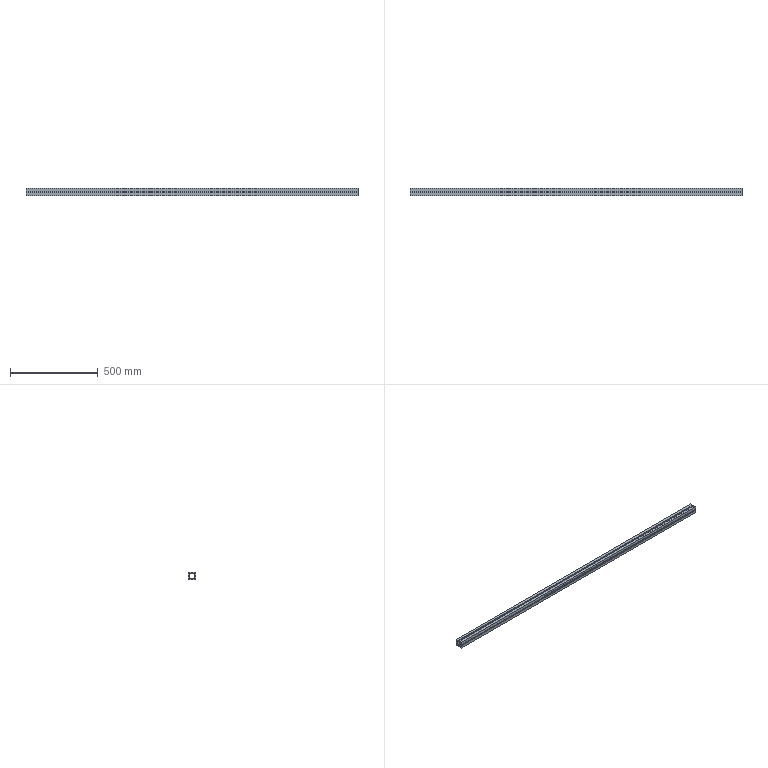Part | SolidWorks | features Extrusion 1 | 1 solid | 42 faces | box 1890 x 40 x 40 mm | volume 1315440 mm3 | plane 42
STEP:
#1=CARTESIAN_POINT('',(1890.,3.,-20.));
#2=VERTEX_POINT('',#1);
#3=CARTESIAN_POINT('',(1890.,20.,-20.));
#4=VERTEX_POINT('',#3);
#5=CARTESIAN_POINT('',(1890.,3.,-20.));
#6=DIRECTION('',(0.,1.,0.));
#7=VECTOR('',#6,1000.);
#8=LINE('',#5,#7);
#9=EDGE_CURVE('',#2,#4,#8,.T.);
#10=ORIENTED_EDGE('',*,*,#9,.T.);
#11=CARTESIAN_POINT('',(1890.,20.,-3.));
#12=VERTEX_POINT('',#11);
#13=CARTESIAN_POINT('',(1890.,20.,-3.));
#14=DIRECTION('',(0.,0.,1.));
#15=VECTOR('',#14,1000.);
#16=LINE('',#13,#15);
#17=EDGE_CURVE('',#4,#12,#16,.T.);
#18=ORIENTED_EDGE('',*,*,#17,.T.);
#19=CARTESIAN_POINT('',(1890.,17.,-3.));
#20=VERTEX_POINT('',#19);
#21=CARTESIAN_POINT('',(1890.,20.,-3.));
#22=DIRECTION('',(0.,-1.,0.));
#23=VECTOR('',#22,1000.);
#24=LINE('',#21,#23);
#25=EDGE_CURVE('',#12,#20,#24,.T.);
#26=ORIENTED_EDGE('',*,*,#25,.T.);
#27=CARTESIAN_POINT('',(1890.,17.,-6.5));
#28=VERTEX_POINT('',#27);
#29=CARTESIAN_POINT('',(1890.,17.,-3.));
#30=DIRECTION('',(0.,0.,-1.));
#31=VECTOR('',#30,1000.);
#32=LINE('',#29,#31);
#33=EDGE_CURVE('',#20,#28,#32,.T.);
#34=ORIENTED_EDGE('',*,*,#33,.T.);
#35=CARTESIAN_POINT('',(1890.,14.,-6.5));
#36=VERTEX_POINT('',#35);
#37=CARTESIAN_POINT('',(1890.,17.,-6.5));
#38=DIRECTION('',(0.,-1.,0.));
#39=VECTOR('',#38,1000.);
#40=LINE('',#37,#39);
#41=EDGE_CURVE('',#28,#36,#40,.T.);
#42=ORIENTED_EDGE('',*,*,#41,.T.);
#43=CARTESIAN_POINT('',(1890.,14.,6.5));
#44=VERTEX_POINT('',#43);
#45=CARTESIAN_POINT('',(1890.,14.,6.5));
#46=DIRECTION('',(0.,0.,1.));
#47=VECTOR('',#46,1000.);
#48=LINE('',#45,#47);
#49=EDGE_CURVE('',#36,#44,#48,.T.);
#50=ORIENTED_EDGE('',*,*,#49,.T.);
#51=CARTESIAN_POINT('',(1890.,17.,6.5));
#52=VERTEX_POINT('',#51);
#53=CARTESIAN_POINT('',(1890.,17.,6.5));
#54=DIRECTION('',(0.,1.,0.));
#55=VECTOR('',#54,1000.);
#56=LINE('',#53,#55);
#57=EDGE_CURVE('',#44,#52,#56,.T.);
#58=ORIENTED_EDGE('',*,*,#57,.T.);
#59=CARTESIAN_POINT('',(1890.,17.,3.));
#60=VERTEX_POINT('',#59);
#61=CARTESIAN_POINT('',(1890.,17.,6.5));
#62=DIRECTION('',(0.,0.,-1.));
#63=VECTOR('',#62,1000.);
#64=LINE('',#61,#63);
#65=EDGE_CURVE('',#52,#60,#64,.T.);
#66=ORIENTED_EDGE('',*,*,#65,.T.);
#67=CARTESIAN_POINT('',(1890.,20.,3.));
#68=VERTEX_POINT('',#67);
#69=CARTESIAN_POINT('',(1890.,20.,3.));
#70=DIRECTION('',(0.,1.,0.));
#71=VECTOR('',#70,1000.);
#72=LINE('',#69,#71);
#73=EDGE_CURVE('',#60,#68,#72,.T.);
#74=ORIENTED_EDGE('',*,*,#73,.T.);
#75=CARTESIAN_POINT('',(1890.,20.,20.));
#76=VERTEX_POINT('',#75);
#77=CARTESIAN_POINT('',(1890.,20.,20.));
#78=DIRECTION('',(0.,0.,1.));
#79=VECTOR('',#78,1000.);
#80=LINE('',#77,#79);
#81=EDGE_CURVE('',#68,#76,#80,.T.);
#82=ORIENTED_EDGE('',*,*,#81,.T.);
#83=CARTESIAN_POINT('',(1890.,3.,20.));
#84=VERTEX_POINT('',#83);
#85=CARTESIAN_POINT('',(1890.,3.,20.));
#86=DIRECTION('',(0.,-1.,0.));
#87=VECTOR('',#86,1000.);
#88=LINE('',#85,#87);
#89=EDGE_CURVE('',#76,#84,#88,.T.);
#90=ORIENTED_EDGE('',*,*,#89,.T.);
#91=CARTESIAN_POINT('',(1890.,3.,17.));
#92=VERTEX_POINT('',#91);
#93=CARTESIAN_POINT('',(1890.,3.,17.));
#94=DIRECTION('',(0.,0.,-1.));
#95=VECTOR('',#94,1000.);
#96=LINE('',#93,#95);
#97=EDGE_CURVE('',#84,#92,#96,.T.);
#98=ORIENTED_EDGE('',*,*,#97,.T.);
#99=CARTESIAN_POINT('',(1890.,6.5,17.));
#100=VERTEX_POINT('',#99);
#101=CARTESIAN_POINT('',(1890.,3.,17.));
#102=DIRECTION('',(0.,1.,0.));
#103=VECTOR('',#102,1000.);
#104=LINE('',#101,#103);
#105=EDGE_CURVE('',#92,#100,#104,.T.);
#106=ORIENTED_EDGE('',*,*,#105,.T.);
#107=CARTESIAN_POINT('',(1890.,6.5,14.));
#108=VERTEX_POINT('',#107);
#109=CARTESIAN_POINT('',(1890.,6.5,14.));
#110=DIRECTION('',(0.,0.,-1.));
#111=VECTOR('',#110,1000.);
#112=LINE('',#109,#111);
#113=EDGE_CURVE('',#100,#108,#112,.T.);
#114=ORIENTED_EDGE('',*,*,#113,.T.);
#115=CARTESIAN_POINT('',(1890.,-6.5,14.));
#116=VERTEX_POINT('',#115);
#117=CARTESIAN_POINT('',(1890.,-6.5,14.));
#118=DIRECTION('',(0.,-1.,0.));
#119=VECTOR('',#118,1000.);
#120=LINE('',#117,#119);
#121=EDGE_CURVE('',#108,#116,#120,.T.);
#122=ORIENTED_EDGE('',*,*,#121,.T.);
#123=CARTESIAN_POINT('',(1890.,-6.5,17.));
#124=VERTEX_POINT('',#123);
#125=CARTESIAN_POINT('',(1890.,-6.5,14.));
#126=DIRECTION('',(0.,0.,1.));
#127=VECTOR('',#126,1000.);
#128=LINE('',#125,#127);
#129=EDGE_CURVE('',#116,#124,#128,.T.);
#130=ORIENTED_EDGE('',*,*,#129,.T.);
#131=CARTESIAN_POINT('',(1890.,-3.,17.));
#132=VERTEX_POINT('',#131);
#133=CARTESIAN_POINT('',(1890.,-6.5,17.));
#134=DIRECTION('',(0.,1.,0.));
#135=VECTOR('',#134,1000.);
#136=LINE('',#133,#135);
#137=EDGE_CURVE('',#124,#132,#136,.T.);
#138=ORIENTED_EDGE('',*,*,#137,.T.);
#139=CARTESIAN_POINT('',(1890.,-3.,20.));
#140=VERTEX_POINT('',#139);
#141=CARTESIAN_POINT('',(1890.,-3.,17.));
#142=DIRECTION('',(0.,0.,1.));
#143=VECTOR('',#142,1000.);
#144=LINE('',#141,#143);
#145=EDGE_CURVE('',#132,#140,#144,.T.);
#146=ORIENTED_EDGE('',*,*,#145,.T.);
#147=CARTESIAN_POINT('',(1890.,-20.,20.));
#148=VERTEX_POINT('',#147);
#149=CARTESIAN_POINT('',(1890.,-20.,20.));
#150=DIRECTION('',(0.,-1.,0.));
#151=VECTOR('',#150,1000.);
#152=LINE('',#149,#151);
#153=EDGE_CURVE('',#140,#148,#152,.T.);
#154=ORIENTED_EDGE('',*,*,#153,.T.);
#155=CARTESIAN_POINT('',(1890.,-20.,3.));
#156=VERTEX_POINT('',#155);
#157=CARTESIAN_POINT('',(1890.,-20.,20.));
#158=DIRECTION('',(0.,0.,-1.));
#159=VECTOR('',#158,1000.);
#160=LINE('',#157,#159);
#161=EDGE_CURVE('',#148,#156,#160,.T.);
#162=ORIENTED_EDGE('',*,*,#161,.T.);
#163=CARTESIAN_POINT('',(1890.,-17.,3.));
#164=VERTEX_POINT('',#163);
#165=CARTESIAN_POINT('',(1890.,-20.,3.));
#166=DIRECTION('',(0.,1.,0.));
#167=VECTOR('',#166,1000.);
#168=LINE('',#165,#167);
#169=EDGE_CURVE('',#156,#164,#168,.T.);
#170=ORIENTED_EDGE('',*,*,#169,.T.);
#171=CARTESIAN_POINT('',(1890.,-17.,6.5));
#172=VERTEX_POINT('',#171);
#173=CARTESIAN_POINT('',(1890.,-17.,6.5));
#174=DIRECTION('',(0.,0.,1.));
#175=VECTOR('',#174,1000.);
#176=LINE('',#173,#175);
#177=EDGE_CURVE('',#164,#172,#176,.T.);
#178=ORIENTED_EDGE('',*,*,#177,.T.);
#179=CARTESIAN_POINT('',(1890.,-14.,6.5));
#180=VERTEX_POINT('',#179);
#181=CARTESIAN_POINT('',(1890.,-17.,6.5));
#182=DIRECTION('',(0.,1.,0.));
#183=VECTOR('',#182,1000.);
#184=LINE('',#181,#183);
#185=EDGE_CURVE('',#172,#180,#184,.T.);
#186=ORIENTED_EDGE('',*,*,#185,.T.);
#187=CARTESIAN_POINT('',(1890.,-14.,-6.5));
#188=VERTEX_POINT('',#187);
#189=CARTESIAN_POINT('',(1890.,-14.,6.5));
#190=DIRECTION('',(0.,0.,-1.));
#191=VECTOR('',#190,1000.);
#192=LINE('',#189,#191);
#193=EDGE_CURVE('',#180,#188,#192,.T.);
#194=ORIENTED_EDGE('',*,*,#193,.T.);
#195=CARTESIAN_POINT('',(1890.,-17.,-6.5));
#196=VERTEX_POINT('',#195);
#197=CARTESIAN_POINT('',(1890.,-17.,-6.5));
#198=DIRECTION('',(0.,-1.,0.));
#199=VECTOR('',#198,1000.);
#200=LINE('',#197,#199);
#201=EDGE_CURVE('',#188,#196,#200,.T.);
#202=ORIENTED_EDGE('',*,*,#201,.T.);
#203=CARTESIAN_POINT('',(1890.,-17.,-3.));
#204=VERTEX_POINT('',#203);
#205=CARTESIAN_POINT('',(1890.,-17.,-3.));
#206=DIRECTION('',(0.,0.,1.));
#207=VECTOR('',#206,1000.);
#208=LINE('',#205,#207);
#209=EDGE_CURVE('',#196,#204,#208,.T.);
#210=ORIENTED_EDGE('',*,*,#209,.T.);
#211=CARTESIAN_POINT('',(1890.,-20.,-3.));
#212=VERTEX_POINT('',#211);
#213=CARTESIAN_POINT('',(1890.,-20.,-3.));
#214=DIRECTION('',(0.,-1.,0.));
#215=VECTOR('',#214,1000.);
#216=LINE('',#213,#215);
#217=EDGE_CURVE('',#204,#212,#216,.T.);
#218=ORIENTED_EDGE('',*,*,#217,.T.);
#219=CARTESIAN_POINT('',(1890.,-20.,-20.));
#220=VERTEX_POINT('',#219);
#221=CARTESIAN_POINT('',(1890.,-20.,-3.));
#222=DIRECTION('',(0.,0.,-1.));
#223=VECTOR('',#222,1000.);
#224=LINE('',#221,#223);
#225=EDGE_CURVE('',#212,#220,#224,.T.);
#226=ORIENTED_EDGE('',*,*,#225,.T.);
#227=CARTESIAN_POINT('',(1890.,-3.,-20.));
#228=VERTEX_POINT('',#227);
#229=CARTESIAN_POINT('',(1890.,-20.,-20.));
#230=DIRECTION('',(0.,1.,0.));
#231=VECTOR('',#230,1000.);
#232=LINE('',#229,#231);
#233=EDGE_CURVE('',#220,#228,#232,.T.);
#234=ORIENTED_EDGE('',*,*,#233,.T.);
#235=CARTESIAN_POINT('',(1890.,-3.,-17.));
#236=VERTEX_POINT('',#235);
#237=CARTESIAN_POINT('',(1890.,-3.,-17.));
#238=DIRECTION('',(0.,0.,1.));
#239=VECTOR('',#238,1000.);
#240=LINE('',#237,#239);
#241=EDGE_CURVE('',#228,#236,#240,.T.);
#242=ORIENTED_EDGE('',*,*,#241,.T.);
#243=CARTESIAN_POINT('',(1890.,-6.5,-17.));
#244=VERTEX_POINT('',#243);
#245=CARTESIAN_POINT('',(1890.,-6.5,-17.));
#246=DIRECTION('',(0.,-1.,0.));
#247=VECTOR('',#246,1000.);
#248=LINE('',#245,#247);
#249=EDGE_CURVE('',#236,#244,#248,.T.);
#250=ORIENTED_EDGE('',*,*,#249,.T.);
#251=CARTESIAN_POINT('',(1890.,-6.5,-14.));
#252=VERTEX_POINT('',#251);
#253=CARTESIAN_POINT('',(1890.,-6.5,-14.));
#254=DIRECTION('',(0.,0.,1.));
#255=VECTOR('',#254,1000.);
#256=LINE('',#253,#255);
#257=EDGE_CURVE('',#244,#252,#256,.T.);
#258=ORIENTED_EDGE('',*,*,#257,.T.);
#259=CARTESIAN_POINT('',(1890.,6.5,-14.));
#260=VERTEX_POINT('',#259);
#261=CARTESIAN_POINT('',(1890.,-6.5,-14.));
#262=DIRECTION('',(0.,1.,0.));
#263=VECTOR('',#262,1000.);
#264=LINE('',#261,#263);
#265=EDGE_CURVE('',#252,#260,#264,.T.);
#266=ORIENTED_EDGE('',*,*,#265,.T.);
#267=CARTESIAN_POINT('',(1890.,6.5,-17.));
#268=VERTEX_POINT('',#267);
#269=CARTESIAN_POINT('',(1890.,6.5,-14.));
#270=DIRECTION('',(0.,0.,-1.));
#271=VECTOR('',#270,1000.);
#272=LINE('',#269,#271);
#273=EDGE_CURVE('',#260,#268,#272,.T.);
#274=ORIENTED_EDGE('',*,*,#273,.T.);
#275=CARTESIAN_POINT('',(1890.,3.,-17.));
#276=VERTEX_POINT('',#275);
#277=CARTESIAN_POINT('',(1890.,3.,-17.));
#278=DIRECTION('',(0.,-1.,0.));
#279=VECTOR('',#278,1000.);
#280=LINE('',#277,#279);
#281=EDGE_CURVE('',#268,#276,#280,.T.);
#282=ORIENTED_EDGE('',*,*,#281,.T.);
#283=CARTESIAN_POINT('',(1890.,3.,-17.));
#284=DIRECTION('',(0.,0.,-1.));
#285=VECTOR('',#284,1000.);
#286=LINE('',#283,#285);
#287=EDGE_CURVE('',#276,#2,#286,.T.);
#288=ORIENTED_EDGE('',*,*,#287,.T.);
#289=EDGE_LOOP('',(#10,#18,#26,#34,#42,#50,#58,#66,#74,#82,#90,#98,#106,#114,#122,#130,#138,#146,#154,#162,#170,#178,#186,#194,#202,#210,#218,#226,#234,#242,#250,#258,#266,#274,#282,#288));
#290=FACE_OUTER_BOUND('',#289,.T.);
#291=CARTESIAN_POINT('',(1890.,-13.,-13.));
#292=VERTEX_POINT('',#291);
#293=CARTESIAN_POINT('',(1890.,13.,-13.));
#294=VERTEX_POINT('',#293);
#295=CARTESIAN_POINT('',(1890.,-13.,-13.));
#296=DIRECTION('',(0.,1.,0.));
#297=VECTOR('',#296,1000.);
#298=LINE('',#295,#297);
#299=EDGE_CURVE('',#292,#294,#298,.T.);
#300=ORIENTED_EDGE('',*,*,#299,.F.);
#301=CARTESIAN_POINT('',(1890.,-13.,13.));
#302=VERTEX_POINT('',#301);
#303=CARTESIAN_POINT('',(1890.,-13.,13.));
#304=DIRECTION('',(0.,0.,-1.));
#305=VECTOR('',#304,1000.);
#306=LINE('',#303,#305);
#307=EDGE_CURVE('',#302,#292,#306,.T.);
#308=ORIENTED_EDGE('',*,*,#307,.F.);
#309=CARTESIAN_POINT('',(1890.,13.,13.));
#310=VERTEX_POINT('',#309);
#311=CARTESIAN_POINT('',(1890.,-13.,13.));
#312=DIRECTION('',(0.,-1.,0.));
#313=VECTOR('',#312,1000.);
#314=LINE('',#311,#313);
#315=EDGE_CURVE('',#310,#302,#314,.T.);
#316=ORIENTED_EDGE('',*,*,#315,.F.);
#317=CARTESIAN_POINT('',(1890.,13.,13.));
#318=DIRECTION('',(0.,0.,1.));
#319=VECTOR('',#318,1000.);
#320=LINE('',#317,#319);
#321=EDGE_CURVE('',#294,#310,#320,.T.);
#322=ORIENTED_EDGE('',*,*,#321,.F.);
#323=EDGE_LOOP('',(#300,#308,#316,#322));
#324=FACE_BOUND('',#323,.T.);
#325=CARTESIAN_POINT('',(1890.,20.,-20.));
#326=DIRECTION('',(-1.,0.,0.));
#327=DIRECTION('',(0.,0.,1.));
#328=AXIS2_PLACEMENT_3D('',#325,#326,#327);
#329=PLANE('',#328);
#330=ADVANCED_FACE('',(#290,#324),#329,.F.);
#331=CARTESIAN_POINT('',(0.,3.,-20.));
#332=VERTEX_POINT('',#331);
#333=CARTESIAN_POINT('',(0.,20.,-20.));
#334=VERTEX_POINT('',#333);
#335=CARTESIAN_POINT('',(0.,3.,-20.));
#336=DIRECTION('',(0.,1.,0.));
#337=VECTOR('',#336,1000.);
#338=LINE('',#335,#337);
#339=EDGE_CURVE('',#332,#334,#338,.T.);
#340=ORIENTED_EDGE('',*,*,#339,.F.);
#341=CARTESIAN_POINT('',(0.,3.,-17.));
#342=VERTEX_POINT('',#341);
#343=CARTESIAN_POINT('',(0.,3.,-17.));
#344=DIRECTION('',(0.,0.,-1.));
#345=VECTOR('',#344,1000.);
#346=LINE('',#343,#345);
#347=EDGE_CURVE('',#342,#332,#346,.T.);
#348=ORIENTED_EDGE('',*,*,#347,.F.);
#349=CARTESIAN_POINT('',(0.,6.5,-17.));
#350=VERTEX_POINT('',#349);
#351=CARTESIAN_POINT('',(0.,3.,-17.));
#352=DIRECTION('',(0.,-1.,0.));
#353=VECTOR('',#352,1000.);
#354=LINE('',#351,#353);
#355=EDGE_CURVE('',#350,#342,#354,.T.);
#356=ORIENTED_EDGE('',*,*,#355,.F.);
#357=CARTESIAN_POINT('',(0.,6.5,-14.));
#358=VERTEX_POINT('',#357);
#359=CARTESIAN_POINT('',(0.,6.5,-14.));
#360=DIRECTION('',(0.,0.,-1.));
#361=VECTOR('',#360,1000.);
#362=LINE('',#359,#361);
#363=EDGE_CURVE('',#358,#350,#362,.T.);
#364=ORIENTED_EDGE('',*,*,#363,.F.);
#365=CARTESIAN_POINT('',(0.,-6.5,-14.));
#366=VERTEX_POINT('',#365);
#367=CARTESIAN_POINT('',(0.,-6.5,-14.));
#368=DIRECTION('',(0.,1.,0.));
#369=VECTOR('',#368,1000.);
#370=LINE('',#367,#369);
#371=EDGE_CURVE('',#366,#358,#370,.T.);
#372=ORIENTED_EDGE('',*,*,#371,.F.);
#373=CARTESIAN_POINT('',(0.,-6.5,-17.));
#374=VERTEX_POINT('',#373);
#375=CARTESIAN_POINT('',(0.,-6.5,-14.));
#376=DIRECTION('',(0.,0.,1.));
#377=VECTOR('',#376,1000.);
#378=LINE('',#375,#377);
#379=EDGE_CURVE('',#374,#366,#378,.T.);
#380=ORIENTED_EDGE('',*,*,#379,.F.);
#381=CARTESIAN_POINT('',(0.,-3.,-17.));
#382=VERTEX_POINT('',#381);
#383=CARTESIAN_POINT('',(0.,-6.5,-17.));
#384=DIRECTION('',(0.,-1.,0.));
#385=VECTOR('',#384,1000.);
#386=LINE('',#383,#385);
#387=EDGE_CURVE('',#382,#374,#386,.T.);
#388=ORIENTED_EDGE('',*,*,#387,.F.);
#389=CARTESIAN_POINT('',(0.,-3.,-20.));
#390=VERTEX_POINT('',#389);
#391=CARTESIAN_POINT('',(0.,-3.,-17.));
#392=DIRECTION('',(0.,0.,1.));
#393=VECTOR('',#392,1000.);
#394=LINE('',#391,#393);
#395=EDGE_CURVE('',#390,#382,#394,.T.);
#396=ORIENTED_EDGE('',*,*,#395,.F.);
#397=CARTESIAN_POINT('',(0.,-20.,-20.));
#398=VERTEX_POINT('',#397);
#399=CARTESIAN_POINT('',(0.,-20.,-20.));
#400=DIRECTION('',(0.,1.,0.));
#401=VECTOR('',#400,1000.);
#402=LINE('',#399,#401);
#403=EDGE_CURVE('',#398,#390,#402,.T.);
#404=ORIENTED_EDGE('',*,*,#403,.F.);
#405=CARTESIAN_POINT('',(0.,-20.,-3.));
#406=VERTEX_POINT('',#405);
#407=CARTESIAN_POINT('',(0.,-20.,-3.));
#408=DIRECTION('',(0.,0.,-1.));
#409=VECTOR('',#408,1000.);
#410=LINE('',#407,#409);
#411=EDGE_CURVE('',#406,#398,#410,.T.);
#412=ORIENTED_EDGE('',*,*,#411,.F.);
#413=CARTESIAN_POINT('',(0.,-17.,-3.));
#414=VERTEX_POINT('',#413);
#415=CARTESIAN_POINT('',(0.,-20.,-3.));
#416=DIRECTION('',(0.,-1.,0.));
#417=VECTOR('',#416,1000.);
#418=LINE('',#415,#417);
#419=EDGE_CURVE('',#414,#406,#418,.T.);
#420=ORIENTED_EDGE('',*,*,#419,.F.);
#421=CARTESIAN_POINT('',(0.,-17.,-6.5));
#422=VERTEX_POINT('',#421);
#423=CARTESIAN_POINT('',(0.,-17.,-3.));
#424=DIRECTION('',(0.,0.,1.));
#425=VECTOR('',#424,1000.);
#426=LINE('',#423,#425);
#427=EDGE_CURVE('',#422,#414,#426,.T.);
#428=ORIENTED_EDGE('',*,*,#427,.F.);
#429=CARTESIAN_POINT('',(0.,-14.,-6.5));
#430=VERTEX_POINT('',#429);
#431=CARTESIAN_POINT('',(0.,-17.,-6.5));
#432=DIRECTION('',(0.,-1.,0.));
#433=VECTOR('',#432,1000.);
#434=LINE('',#431,#433);
#435=EDGE_CURVE('',#430,#422,#434,.T.);
#436=ORIENTED_EDGE('',*,*,#435,.F.);
#437=CARTESIAN_POINT('',(0.,-14.,6.5));
#438=VERTEX_POINT('',#437);
#439=CARTESIAN_POINT('',(0.,-14.,6.5));
#440=DIRECTION('',(0.,0.,-1.));
#441=VECTOR('',#440,1000.);
#442=LINE('',#439,#441);
#443=EDGE_CURVE('',#438,#430,#442,.T.);
#444=ORIENTED_EDGE('',*,*,#443,.F.);
#445=CARTESIAN_POINT('',(0.,-17.,6.5));
#446=VERTEX_POINT('',#445);
#447=CARTESIAN_POINT('',(0.,-17.,6.5));
#448=DIRECTION('',(0.,1.,0.));
#449=VECTOR('',#448,1000.);
#450=LINE('',#447,#449);
#451=EDGE_CURVE('',#446,#438,#450,.T.);
#452=ORIENTED_EDGE('',*,*,#451,.F.);
#453=CARTESIAN_POINT('',(0.,-17.,3.));
#454=VERTEX_POINT('',#453);
#455=CARTESIAN_POINT('',(0.,-17.,6.5));
#456=DIRECTION('',(0.,0.,1.));
#457=VECTOR('',#456,1000.);
#458=LINE('',#455,#457);
#459=EDGE_CURVE('',#454,#446,#458,.T.);
#460=ORIENTED_EDGE('',*,*,#459,.F.);
#461=CARTESIAN_POINT('',(0.,-20.,3.));
#462=VERTEX_POINT('',#461);
#463=CARTESIAN_POINT('',(0.,-20.,3.));
#464=DIRECTION('',(0.,1.,0.));
#465=VECTOR('',#464,1000.);
#466=LINE('',#463,#465);
#467=EDGE_CURVE('',#462,#454,#466,.T.);
#468=ORIENTED_EDGE('',*,*,#467,.F.);
#469=CARTESIAN_POINT('',(0.,-20.,20.));
#470=VERTEX_POINT('',#469);
#471=CARTESIAN_POINT('',(0.,-20.,20.));
#472=DIRECTION('',(0.,0.,-1.));
#473=VECTOR('',#472,1000.);
#474=LINE('',#471,#473);
#475=EDGE_CURVE('',#470,#462,#474,.T.);
#476=ORIENTED_EDGE('',*,*,#475,.F.);
#477=CARTESIAN_POINT('',(0.,-3.,20.));
#478=VERTEX_POINT('',#477);
#479=CARTESIAN_POINT('',(0.,-20.,20.));
#480=DIRECTION('',(0.,-1.,0.));
#481=VECTOR('',#480,1000.);
#482=LINE('',#479,#481);
#483=EDGE_CURVE('',#478,#470,#482,.T.);
#484=ORIENTED_EDGE('',*,*,#483,.F.);
#485=CARTESIAN_POINT('',(0.,-3.,17.));
#486=VERTEX_POINT('',#485);
#487=CARTESIAN_POINT('',(0.,-3.,17.));
#488=DIRECTION('',(0.,0.,1.));
#489=VECTOR('',#488,1000.);
#490=LINE('',#487,#489);
#491=EDGE_CURVE('',#486,#478,#490,.T.);
#492=ORIENTED_EDGE('',*,*,#491,.F.);
#493=CARTESIAN_POINT('',(0.,-6.5,17.));
#494=VERTEX_POINT('',#493);
#495=CARTESIAN_POINT('',(0.,-6.5,17.));
#496=DIRECTION('',(0.,1.,0.));
#497=VECTOR('',#496,1000.);
#498=LINE('',#495,#497);
#499=EDGE_CURVE('',#494,#486,#498,.T.);
#500=ORIENTED_EDGE('',*,*,#499,.F.);
#501=CARTESIAN_POINT('',(0.,-6.5,14.));
#502=VERTEX_POINT('',#501);
#503=CARTESIAN_POINT('',(0.,-6.5,14.));
#504=DIRECTION('',(0.,0.,1.));
#505=VECTOR('',#504,1000.);
#506=LINE('',#503,#505);
#507=EDGE_CURVE('',#502,#494,#506,.T.);
#508=ORIENTED_EDGE('',*,*,#507,.F.);
#509=CARTESIAN_POINT('',(0.,6.5,14.));
#510=VERTEX_POINT('',#509);
#511=CARTESIAN_POINT('',(0.,-6.5,14.));
#512=DIRECTION('',(0.,-1.,0.));
#513=VECTOR('',#512,1000.);
#514=LINE('',#511,#513);
#515=EDGE_CURVE('',#510,#502,#514,.T.);
#516=ORIENTED_EDGE('',*,*,#515,.F.);
#517=CARTESIAN_POINT('',(0.,6.5,17.));
#518=VERTEX_POINT('',#517);
#519=CARTESIAN_POINT('',(0.,6.5,14.));
#520=DIRECTION('',(0.,0.,-1.));
#521=VECTOR('',#520,1000.);
#522=LINE('',#519,#521);
#523=EDGE_CURVE('',#518,#510,#522,.T.);
#524=ORIENTED_EDGE('',*,*,#523,.F.);
#525=CARTESIAN_POINT('',(0.,3.,17.));
#526=VERTEX_POINT('',#525);
#527=CARTESIAN_POINT('',(0.,3.,17.));
#528=DIRECTION('',(0.,1.,0.));
#529=VECTOR('',#528,1000.);
#530=LINE('',#527,#529);
#531=EDGE_CURVE('',#526,#518,#530,.T.);
#532=ORIENTED_EDGE('',*,*,#531,.F.);
#533=CARTESIAN_POINT('',(0.,3.,20.));
#534=VERTEX_POINT('',#533);
#535=CARTESIAN_POINT('',(0.,3.,17.));
#536=DIRECTION('',(0.,0.,-1.));
#537=VECTOR('',#536,1000.);
#538=LINE('',#535,#537);
#539=EDGE_CURVE('',#534,#526,#538,.T.);
#540=ORIENTED_EDGE('',*,*,#539,.F.);
#541=CARTESIAN_POINT('',(0.,20.,20.));
#542=VERTEX_POINT('',#541);
#543=CARTESIAN_POINT('',(0.,3.,20.));
#544=DIRECTION('',(0.,-1.,0.));
#545=VECTOR('',#544,1000.);
#546=LINE('',#543,#545);
#547=EDGE_CURVE('',#542,#534,#546,.T.);
#548=ORIENTED_EDGE('',*,*,#547,.F.);
#549=CARTESIAN_POINT('',(0.,20.,3.));
#550=VERTEX_POINT('',#549);
#551=CARTESIAN_POINT('',(0.,20.,20.));
#552=DIRECTION('',(0.,0.,1.));
#553=VECTOR('',#552,1000.);
#554=LINE('',#551,#553);
#555=EDGE_CURVE('',#550,#542,#554,.T.);
#556=ORIENTED_EDGE('',*,*,#555,.F.);
#557=CARTESIAN_POINT('',(0.,17.,3.));
#558=VERTEX_POINT('',#557);
#559=CARTESIAN_POINT('',(0.,20.,3.));
#560=DIRECTION('',(0.,1.,0.));
#561=VECTOR('',#560,1000.);
#562=LINE('',#559,#561);
#563=EDGE_CURVE('',#558,#550,#562,.T.);
#564=ORIENTED_EDGE('',*,*,#563,.F.);
#565=CARTESIAN_POINT('',(0.,17.,6.5));
#566=VERTEX_POINT('',#565);
#567=CARTESIAN_POINT('',(0.,17.,6.5));
#568=DIRECTION('',(0.,0.,-1.));
#569=VECTOR('',#568,1000.);
#570=LINE('',#567,#569);
#571=EDGE_CURVE('',#566,#558,#570,.T.);
#572=ORIENTED_EDGE('',*,*,#571,.F.);
#573=CARTESIAN_POINT('',(0.,14.,6.5));
#574=VERTEX_POINT('',#573);
#575=CARTESIAN_POINT('',(0.,17.,6.5));
#576=DIRECTION('',(0.,1.,0.));
#577=VECTOR('',#576,1000.);
#578=LINE('',#575,#577);
#579=EDGE_CURVE('',#574,#566,#578,.T.);
#580=ORIENTED_EDGE('',*,*,#579,.F.);
#581=CARTESIAN_POINT('',(0.,14.,-6.5));
#582=VERTEX_POINT('',#581);
#583=CARTESIAN_POINT('',(0.,14.,6.5));
#584=DIRECTION('',(0.,0.,1.));
#585=VECTOR('',#584,1000.);
#586=LINE('',#583,#585);
#587=EDGE_CURVE('',#582,#574,#586,.T.);
#588=ORIENTED_EDGE('',*,*,#587,.F.);
#589=CARTESIAN_POINT('',(0.,17.,-6.5));
#590=VERTEX_POINT('',#589);
#591=CARTESIAN_POINT('',(0.,17.,-6.5));
#592=DIRECTION('',(0.,-1.,0.));
#593=VECTOR('',#592,1000.);
#594=LINE('',#591,#593);
#595=EDGE_CURVE('',#590,#582,#594,.T.);
#596=ORIENTED_EDGE('',*,*,#595,.F.);
#597=CARTESIAN_POINT('',(0.,17.,-3.));
#598=VERTEX_POINT('',#597);
#599=CARTESIAN_POINT('',(0.,17.,-3.));
#600=DIRECTION('',(0.,0.,-1.));
#601=VECTOR('',#600,1000.);
#602=LINE('',#599,#601);
#603=EDGE_CURVE('',#598,#590,#602,.T.);
#604=ORIENTED_EDGE('',*,*,#603,.F.);
#605=CARTESIAN_POINT('',(0.,20.,-3.));
#606=VERTEX_POINT('',#605);
#607=CARTESIAN_POINT('',(0.,20.,-3.));
#608=DIRECTION('',(0.,-1.,0.));
#609=VECTOR('',#608,1000.);
#610=LINE('',#607,#609);
#611=EDGE_CURVE('',#606,#598,#610,.T.);
#612=ORIENTED_EDGE('',*,*,#611,.F.);
#613=CARTESIAN_POINT('',(0.,20.,-3.));
#614=DIRECTION('',(0.,0.,1.));
#615=VECTOR('',#614,1000.);
#616=LINE('',#613,#615);
#617=EDGE_CURVE('',#334,#606,#616,.T.);
#618=ORIENTED_EDGE('',*,*,#617,.F.);
#619=EDGE_LOOP('',(#340,#348,#356,#364,#372,#380,#388,#396,#404,#412,#420,#428,#436,#444,#452,#460,#468,#476,#484,#492,#500,#508,#516,#524,#532,#540,#548,#556,#564,#572,#580,#588,#596,#604,#612,#618));
#620=FACE_OUTER_BOUND('',#619,.T.);
#621=CARTESIAN_POINT('',(0.,-13.,13.));
#622=VERTEX_POINT('',#621);
#623=CARTESIAN_POINT('',(0.,-13.,-13.));
#624=VERTEX_POINT('',#623);
#625=CARTESIAN_POINT('',(0.,-13.,13.));
#626=DIRECTION('',(0.,0.,-1.));
#627=VECTOR('',#626,1000.);
#628=LINE('',#625,#627);
#629=EDGE_CURVE('',#622,#624,#628,.T.);
#630=ORIENTED_EDGE('',*,*,#629,.T.);
#631=CARTESIAN_POINT('',(0.,13.,-13.));
#632=VERTEX_POINT('',#631);
#633=CARTESIAN_POINT('',(0.,-13.,-13.));
#634=DIRECTION('',(0.,1.,0.));
#635=VECTOR('',#634,1000.);
#636=LINE('',#633,#635);
#637=EDGE_CURVE('',#624,#632,#636,.T.);
#638=ORIENTED_EDGE('',*,*,#637,.T.);
#639=CARTESIAN_POINT('',(0.,13.,13.));
#640=VERTEX_POINT('',#639);
#641=CARTESIAN_POINT('',(0.,13.,13.));
#642=DIRECTION('',(0.,0.,1.));
#643=VECTOR('',#642,1000.);
#644=LINE('',#641,#643);
#645=EDGE_CURVE('',#632,#640,#644,.T.);
#646=ORIENTED_EDGE('',*,*,#645,.T.);
#647=CARTESIAN_POINT('',(0.,-13.,13.));
#648=DIRECTION('',(0.,-1.,0.));
#649=VECTOR('',#648,1000.);
#650=LINE('',#647,#649);
#651=EDGE_CURVE('',#640,#622,#650,.T.);
#652=ORIENTED_EDGE('',*,*,#651,.T.);
#653=EDGE_LOOP('',(#630,#638,#646,#652));
#654=FACE_BOUND('',#653,.T.);
#655=CARTESIAN_POINT('',(0.,20.,-20.));
#656=DIRECTION('',(-1.,0.,0.));
#657=DIRECTION('',(0.,0.,1.));
#658=AXIS2_PLACEMENT_3D('',#655,#656,#657);
#659=PLANE('',#658);
#660=ADVANCED_FACE('',(#620,#654),#659,.T.);
#661=ORIENTED_EDGE('',*,*,#339,.T.);
#662=CARTESIAN_POINT('',(1890.,20.,-20.));
#663=DIRECTION('',(-1.,0.,0.));
#664=VECTOR('',#663,1000.);
#665=LINE('',#662,#664);
#666=EDGE_CURVE('',#4,#334,#665,.T.);
#667=ORIENTED_EDGE('',*,*,#666,.F.);
#668=ORIENTED_EDGE('',*,*,#9,.F.);
#669=CARTESIAN_POINT('',(1890.,3.,-20.));
#670=DIRECTION('',(-1.,0.,0.));
#671=VECTOR('',#670,1000.);
#672=LINE('',#669,#671);
#673=EDGE_CURVE('',#2,#332,#672,.T.);
#674=ORIENTED_EDGE('',*,*,#673,.T.);
#675=EDGE_LOOP('',(#661,#667,#668,#674));
#676=FACE_OUTER_BOUND('',#675,.T.);
#677=CARTESIAN_POINT('',(1890.,3.,-20.));
#678=DIRECTION('',(0.,0.,1.));
#679=DIRECTION('',(0.,-1.,0.));
#680=AXIS2_PLACEMENT_3D('',#677,#678,#679);
#681=PLANE('',#680);
#682=ADVANCED_FACE('',(#676),#681,.F.);
#683=ORIENTED_EDGE('',*,*,#617,.T.);
#684=CARTESIAN_POINT('',(1890.,20.,-3.));
#685=DIRECTION('',(-1.,0.,0.));
#686=VECTOR('',#685,1000.);
#687=LINE('',#684,#686);
#688=EDGE_CURVE('',#12,#606,#687,.T.);
#689=ORIENTED_EDGE('',*,*,#688,.F.);
#690=ORIENTED_EDGE('',*,*,#17,.F.);
#691=ORIENTED_EDGE('',*,*,#666,.T.);
#692=EDGE_LOOP('',(#683,#689,#690,#691));
#693=FACE_OUTER_BOUND('',#692,.T.);
#694=CARTESIAN_POINT('',(1890.,20.,-3.));
#695=DIRECTION('',(0.,-1.,0.));
#696=DIRECTION('',(0.,0.,-1.));
#697=AXIS2_PLACEMENT_3D('',#694,#695,#696);
#698=PLANE('',#697);
#699=ADVANCED_FACE('',(#693),#698,.F.);
#700=ORIENTED_EDGE('',*,*,#611,.T.);
#701=CARTESIAN_POINT('',(1890.,17.,-3.));
#702=DIRECTION('',(-1.,0.,0.));
#703=VECTOR('',#702,1000.);
#704=LINE('',#701,#703);
#705=EDGE_CURVE('',#20,#598,#704,.T.);
#706=ORIENTED_EDGE('',*,*,#705,.F.);
#707=ORIENTED_EDGE('',*,*,#25,.F.);
#708=ORIENTED_EDGE('',*,*,#688,.T.);
#709=EDGE_LOOP('',(#700,#706,#707,#708));
#710=FACE_OUTER_BOUND('',#709,.T.);
#711=CARTESIAN_POINT('',(1890.,20.,-3.));
#712=DIRECTION('',(0.,0.,-1.));
#713=DIRECTION('',(0.,1.,0.));
#714=AXIS2_PLACEMENT_3D('',#711,#712,#713);
#715=PLANE('',#714);
#716=ADVANCED_FACE('',(#710),#715,.F.);
#717=ORIENTED_EDGE('',*,*,#603,.T.);
#718=CARTESIAN_POINT('',(1890.,17.,-6.5));
#719=DIRECTION('',(-1.,0.,0.));
#720=VECTOR('',#719,1000.);
#721=LINE('',#718,#720);
#722=EDGE_CURVE('',#28,#590,#721,.T.);
#723=ORIENTED_EDGE('',*,*,#722,.F.);
#724=ORIENTED_EDGE('',*,*,#33,.F.);
#725=ORIENTED_EDGE('',*,*,#705,.T.);
#726=EDGE_LOOP('',(#717,#723,#724,#725));
#727=FACE_OUTER_BOUND('',#726,.T.);
#728=CARTESIAN_POINT('',(1890.,17.,-3.));
#729=DIRECTION('',(0.,1.,0.));
#730=DIRECTION('',(0.,0.,1.));
#731=AXIS2_PLACEMENT_3D('',#728,#729,#730);
#732=PLANE('',#731);
#733=ADVANCED_FACE('',(#727),#732,.F.);
#734=ORIENTED_EDGE('',*,*,#595,.T.);
#735=CARTESIAN_POINT('',(1890.,14.,-6.5));
#736=DIRECTION('',(-1.,0.,0.));
#737=VECTOR('',#736,1000.);
#738=LINE('',#735,#737);
#739=EDGE_CURVE('',#36,#582,#738,.T.);
#740=ORIENTED_EDGE('',*,*,#739,.F.);
#741=ORIENTED_EDGE('',*,*,#41,.F.);
#742=ORIENTED_EDGE('',*,*,#722,.T.);
#743=EDGE_LOOP('',(#734,#740,#741,#742));
#744=FACE_OUTER_BOUND('',#743,.T.);
#745=CARTESIAN_POINT('',(1890.,17.,-6.5));
#746=DIRECTION('',(0.,0.,-1.));
#747=DIRECTION('',(-1.,0.,0.));
#748=AXIS2_PLACEMENT_3D('',#745,#746,#747);
#749=PLANE('',#748);
#750=ADVANCED_FACE('',(#744),#749,.F.);
#751=ORIENTED_EDGE('',*,*,#587,.T.);
#752=CARTESIAN_POINT('',(1890.,14.,6.5));
#753=DIRECTION('',(-1.,0.,0.));
#754=VECTOR('',#753,1000.);
#755=LINE('',#752,#754);
#756=EDGE_CURVE('',#44,#574,#755,.T.);
#757=ORIENTED_EDGE('',*,*,#756,.F.);
#758=ORIENTED_EDGE('',*,*,#49,.F.);
#759=ORIENTED_EDGE('',*,*,#739,.T.);
#760=EDGE_LOOP('',(#751,#757,#758,#759));
#761=FACE_OUTER_BOUND('',#760,.T.);
#762=CARTESIAN_POINT('',(1890.,14.,6.5));
#763=DIRECTION('',(0.,-1.,0.));
#764=DIRECTION('',(0.,0.,-1.));
#765=AXIS2_PLACEMENT_3D('',#762,#763,#764);
#766=PLANE('',#765);
#767=ADVANCED_FACE('',(#761),#766,.F.);
#768=ORIENTED_EDGE('',*,*,#579,.T.);
#769=CARTESIAN_POINT('',(1890.,17.,6.5));
#770=DIRECTION('',(-1.,0.,0.));
#771=VECTOR('',#770,1000.);
#772=LINE('',#769,#771);
#773=EDGE_CURVE('',#52,#566,#772,.T.);
#774=ORIENTED_EDGE('',*,*,#773,.F.);
#775=ORIENTED_EDGE('',*,*,#57,.F.);
#776=ORIENTED_EDGE('',*,*,#756,.T.);
#777=EDGE_LOOP('',(#768,#774,#775,#776));
#778=FACE_OUTER_BOUND('',#777,.T.);
#779=CARTESIAN_POINT('',(1890.,17.,6.5));
#780=DIRECTION('',(0.,0.,1.));
#781=DIRECTION('',(1.,0.,0.));
#782=AXIS2_PLACEMENT_3D('',#779,#780,#781);
#783=PLANE('',#782);
#784=ADVANCED_FACE('',(#778),#783,.F.);
#785=ORIENTED_EDGE('',*,*,#571,.T.);
#786=CARTESIAN_POINT('',(1890.,17.,3.));
#787=DIRECTION('',(-1.,0.,0.));
#788=VECTOR('',#787,1000.);
#789=LINE('',#786,#788);
#790=EDGE_CURVE('',#60,#558,#789,.T.);
#791=ORIENTED_EDGE('',*,*,#790,.F.);
#792=ORIENTED_EDGE('',*,*,#65,.F.);
#793=ORIENTED_EDGE('',*,*,#773,.T.);
#794=EDGE_LOOP('',(#785,#791,#792,#793));
#795=FACE_OUTER_BOUND('',#794,.T.);
#796=CARTESIAN_POINT('',(1890.,17.,6.5));
#797=DIRECTION('',(0.,1.,0.));
#798=DIRECTION('',(0.,0.,1.));
#799=AXIS2_PLACEMENT_3D('',#796,#797,#798);
#800=PLANE('',#799);
#801=ADVANCED_FACE('',(#795),#800,.F.);
#802=ORIENTED_EDGE('',*,*,#563,.T.);
#803=CARTESIAN_POINT('',(1890.,20.,3.));
#804=DIRECTION('',(-1.,0.,0.));
#805=VECTOR('',#804,1000.);
#806=LINE('',#803,#805);
#807=EDGE_CURVE('',#68,#550,#806,.T.);
#808=ORIENTED_EDGE('',*,*,#807,.F.);
#809=ORIENTED_EDGE('',*,*,#73,.F.);
#810=ORIENTED_EDGE('',*,*,#790,.T.);
#811=EDGE_LOOP('',(#802,#808,#809,#810));
#812=FACE_OUTER_BOUND('',#811,.T.);
#813=CARTESIAN_POINT('',(1890.,20.,3.));
#814=DIRECTION('',(0.,0.,1.));
#815=DIRECTION('',(0.,-1.,0.));
#816=AXIS2_PLACEMENT_3D('',#813,#814,#815);
#817=PLANE('',#816);
#818=ADVANCED_FACE('',(#812),#817,.F.);
#819=ORIENTED_EDGE('',*,*,#555,.T.);
#820=CARTESIAN_POINT('',(1890.,20.,20.));
#821=DIRECTION('',(-1.,0.,0.));
#822=VECTOR('',#821,1000.);
#823=LINE('',#820,#822);
#824=EDGE_CURVE('',#76,#542,#823,.T.);
#825=ORIENTED_EDGE('',*,*,#824,.F.);
#826=ORIENTED_EDGE('',*,*,#81,.F.);
#827=ORIENTED_EDGE('',*,*,#807,.T.);
#828=EDGE_LOOP('',(#819,#825,#826,#827));
#829=FACE_OUTER_BOUND('',#828,.T.);
#830=CARTESIAN_POINT('',(1890.,20.,20.));
#831=DIRECTION('',(0.,-1.,0.));
#832=DIRECTION('',(0.,0.,-1.));
#833=AXIS2_PLACEMENT_3D('',#830,#831,#832);
#834=PLANE('',#833);
#835=ADVANCED_FACE('',(#829),#834,.F.);
#836=ORIENTED_EDGE('',*,*,#547,.T.);
#837=CARTESIAN_POINT('',(1890.,3.,20.));
#838=DIRECTION('',(-1.,0.,0.));
#839=VECTOR('',#838,1000.);
#840=LINE('',#837,#839);
#841=EDGE_CURVE('',#84,#534,#840,.T.);
#842=ORIENTED_EDGE('',*,*,#841,.F.);
#843=ORIENTED_EDGE('',*,*,#89,.F.);
#844=ORIENTED_EDGE('',*,*,#824,.T.);
#845=EDGE_LOOP('',(#836,#842,#843,#844));
#846=FACE_OUTER_BOUND('',#845,.T.);
#847=CARTESIAN_POINT('',(1890.,3.,20.));
#848=DIRECTION('',(0.,0.,-1.));
#849=DIRECTION('',(0.,1.,0.));
#850=AXIS2_PLACEMENT_3D('',#847,#848,#849);
#851=PLANE('',#850);
#852=ADVANCED_FACE('',(#846),#851,.F.);
#853=ORIENTED_EDGE('',*,*,#539,.T.);
#854=CARTESIAN_POINT('',(1890.,3.,17.));
#855=DIRECTION('',(-1.,0.,0.));
#856=VECTOR('',#855,1000.);
#857=LINE('',#854,#856);
#858=EDGE_CURVE('',#92,#526,#857,.T.);
#859=ORIENTED_EDGE('',*,*,#858,.F.);
#860=ORIENTED_EDGE('',*,*,#97,.F.);
#861=ORIENTED_EDGE('',*,*,#841,.T.);
#862=EDGE_LOOP('',(#853,#859,#860,#861));
#863=FACE_OUTER_BOUND('',#862,.T.);
#864=CARTESIAN_POINT('',(1890.,3.,17.));
#865=DIRECTION('',(0.,1.,0.));
#866=DIRECTION('',(0.,0.,1.));
#867=AXIS2_PLACEMENT_3D('',#864,#865,#866);
#868=PLANE('',#867);
#869=ADVANCED_FACE('',(#863),#868,.F.);
#870=ORIENTED_EDGE('',*,*,#531,.T.);
#871=CARTESIAN_POINT('',(1890.,6.5,17.));
#872=DIRECTION('',(-1.,0.,0.));
#873=VECTOR('',#872,1000.);
#874=LINE('',#871,#873);
#875=EDGE_CURVE('',#100,#518,#874,.T.);
#876=ORIENTED_EDGE('',*,*,#875,.F.);
#877=ORIENTED_EDGE('',*,*,#105,.F.);
#878=ORIENTED_EDGE('',*,*,#858,.T.);
#879=EDGE_LOOP('',(#870,#876,#877,#878));
#880=FACE_OUTER_BOUND('',#879,.T.);
#881=CARTESIAN_POINT('',(1890.,3.,17.));
#882=DIRECTION('',(0.,0.,1.));
#883=DIRECTION('',(1.,0.,0.));
#884=AXIS2_PLACEMENT_3D('',#881,#882,#883);
#885=PLANE('',#884);
#886=ADVANCED_FACE('',(#880),#885,.F.);
#887=ORIENTED_EDGE('',*,*,#523,.T.);
#888=CARTESIAN_POINT('',(1890.,6.5,14.));
#889=DIRECTION('',(-1.,0.,0.));
#890=VECTOR('',#889,1000.);
#891=LINE('',#888,#890);
#892=EDGE_CURVE('',#108,#510,#891,.T.);
#893=ORIENTED_EDGE('',*,*,#892,.F.);
#894=ORIENTED_EDGE('',*,*,#113,.F.);
#895=ORIENTED_EDGE('',*,*,#875,.T.);
#896=EDGE_LOOP('',(#887,#893,#894,#895));
#897=FACE_OUTER_BOUND('',#896,.T.);
#898=CARTESIAN_POINT('',(1890.,6.5,14.));
#899=DIRECTION('',(0.,1.,0.));
#900=DIRECTION('',(0.,0.,1.));
#901=AXIS2_PLACEMENT_3D('',#898,#899,#900);
#902=PLANE('',#901);
#903=ADVANCED_FACE('',(#897),#902,.F.);
#904=ORIENTED_EDGE('',*,*,#515,.T.);
#905=CARTESIAN_POINT('',(1890.,-6.5,14.));
#906=DIRECTION('',(-1.,0.,0.));
#907=VECTOR('',#906,1000.);
#908=LINE('',#905,#907);
#909=EDGE_CURVE('',#116,#502,#908,.T.);
#910=ORIENTED_EDGE('',*,*,#909,.F.);
#911=ORIENTED_EDGE('',*,*,#121,.F.);
#912=ORIENTED_EDGE('',*,*,#892,.T.);
#913=EDGE_LOOP('',(#904,#910,#911,#912));
#914=FACE_OUTER_BOUND('',#913,.T.);
#915=CARTESIAN_POINT('',(1890.,-6.5,14.));
#916=DIRECTION('',(0.,0.,-1.));
#917=DIRECTION('',(-1.,0.,0.));
#918=AXIS2_PLACEMENT_3D('',#915,#916,#917);
#919=PLANE('',#918);
#920=ADVANCED_FACE('',(#914),#919,.F.);
#921=ORIENTED_EDGE('',*,*,#507,.T.);
#922=CARTESIAN_POINT('',(1890.,-6.5,17.));
#923=DIRECTION('',(-1.,0.,0.));
#924=VECTOR('',#923,1000.);
#925=LINE('',#922,#924);
#926=EDGE_CURVE('',#124,#494,#925,.T.);
#927=ORIENTED_EDGE('',*,*,#926,.F.);
#928=ORIENTED_EDGE('',*,*,#129,.F.);
#929=ORIENTED_EDGE('',*,*,#909,.T.);
#930=EDGE_LOOP('',(#921,#927,#928,#929));
#931=FACE_OUTER_BOUND('',#930,.T.);
#932=CARTESIAN_POINT('',(1890.,-6.5,14.));
#933=DIRECTION('',(0.,-1.,0.));
#934=DIRECTION('',(0.,0.,-1.));
#935=AXIS2_PLACEMENT_3D('',#932,#933,#934);
#936=PLANE('',#935);
#937=ADVANCED_FACE('',(#931),#936,.F.);
#938=ORIENTED_EDGE('',*,*,#499,.T.);
#939=CARTESIAN_POINT('',(1890.,-3.,17.));
#940=DIRECTION('',(-1.,0.,0.));
#941=VECTOR('',#940,1000.);
#942=LINE('',#939,#941);
#943=EDGE_CURVE('',#132,#486,#942,.T.);
#944=ORIENTED_EDGE('',*,*,#943,.F.);
#945=ORIENTED_EDGE('',*,*,#137,.F.);
#946=ORIENTED_EDGE('',*,*,#926,.T.);
#947=EDGE_LOOP('',(#938,#944,#945,#946));
#948=FACE_OUTER_BOUND('',#947,.T.);
#949=CARTESIAN_POINT('',(1890.,-6.5,17.));
#950=DIRECTION('',(0.,0.,1.));
#951=DIRECTION('',(0.,-1.,0.));
#952=AXIS2_PLACEMENT_3D('',#949,#950,#951);
#953=PLANE('',#952);
#954=ADVANCED_FACE('',(#948),#953,.F.);
#955=ORIENTED_EDGE('',*,*,#491,.T.);
#956=CARTESIAN_POINT('',(1890.,-3.,20.));
#957=DIRECTION('',(-1.,0.,0.));
#958=VECTOR('',#957,1000.);
#959=LINE('',#956,#958);
#960=EDGE_CURVE('',#140,#478,#959,.T.);
#961=ORIENTED_EDGE('',*,*,#960,.F.);
#962=ORIENTED_EDGE('',*,*,#145,.F.);
#963=ORIENTED_EDGE('',*,*,#943,.T.);
#964=EDGE_LOOP('',(#955,#961,#962,#963));
#965=FACE_OUTER_BOUND('',#964,.T.);
#966=CARTESIAN_POINT('',(1890.,-3.,17.));
#967=DIRECTION('',(0.,-1.,0.));
#968=DIRECTION('',(0.,0.,-1.));
#969=AXIS2_PLACEMENT_3D('',#966,#967,#968);
#970=PLANE('',#969);
#971=ADVANCED_FACE('',(#965),#970,.F.);
#972=ORIENTED_EDGE('',*,*,#483,.T.);
#973=CARTESIAN_POINT('',(1890.,-20.,20.));
#974=DIRECTION('',(-1.,0.,0.));
#975=VECTOR('',#974,1000.);
#976=LINE('',#973,#975);
#977=EDGE_CURVE('',#148,#470,#976,.T.);
#978=ORIENTED_EDGE('',*,*,#977,.F.);
#979=ORIENTED_EDGE('',*,*,#153,.F.);
#980=ORIENTED_EDGE('',*,*,#960,.T.);
#981=EDGE_LOOP('',(#972,#978,#979,#980));
#982=FACE_OUTER_BOUND('',#981,.T.);
#983=CARTESIAN_POINT('',(1890.,-20.,20.));
#984=DIRECTION('',(0.,0.,-1.));
#985=DIRECTION('',(0.,1.,0.));
#986=AXIS2_PLACEMENT_3D('',#983,#984,#985);
#987=PLANE('',#986);
#988=ADVANCED_FACE('',(#982),#987,.F.);
#989=ORIENTED_EDGE('',*,*,#475,.T.);
#990=CARTESIAN_POINT('',(1890.,-20.,3.));
#991=DIRECTION('',(-1.,0.,0.));
#992=VECTOR('',#991,1000.);
#993=LINE('',#990,#992);
#994=EDGE_CURVE('',#156,#462,#993,.T.);
#995=ORIENTED_EDGE('',*,*,#994,.F.);
#996=ORIENTED_EDGE('',*,*,#161,.F.);
#997=ORIENTED_EDGE('',*,*,#977,.T.);
#998=EDGE_LOOP('',(#989,#995,#996,#997));
#999=FACE_OUTER_BOUND('',#998,.T.);
#1000=CARTESIAN_POINT('',(1890.,-20.,20.));
#1001=DIRECTION('',(0.,1.,0.));
#1002=DIRECTION('',(0.,0.,1.));
#1003=AXIS2_PLACEMENT_3D('',#1000,#1001,#1002);
#1004=PLANE('',#1003);
#1005=ADVANCED_FACE('',(#999),#1004,.F.);
#1006=ORIENTED_EDGE('',*,*,#467,.T.);
#1007=CARTESIAN_POINT('',(1890.,-17.,3.));
#1008=DIRECTION('',(-1.,0.,0.));
#1009=VECTOR('',#1008,1000.);
#1010=LINE('',#1007,#1009);
#1011=EDGE_CURVE('',#164,#454,#1010,.T.);
#1012=ORIENTED_EDGE('',*,*,#1011,.F.);
#1013=ORIENTED_EDGE('',*,*,#169,.F.);
#1014=ORIENTED_EDGE('',*,*,#994,.T.);
#1015=EDGE_LOOP('',(#1006,#1012,#1013,#1014));
#1016=FACE_OUTER_BOUND('',#1015,.T.);
#1017=CARTESIAN_POINT('',(1890.,-20.,3.));
#1018=DIRECTION('',(0.,0.,1.));
#1019=DIRECTION('',(0.,-1.,0.));
#1020=AXIS2_PLACEMENT_3D('',#1017,#1018,#1019);
#1021=PLANE('',#1020);
#1022=ADVANCED_FACE('',(#1016),#1021,.F.);
#1023=ORIENTED_EDGE('',*,*,#459,.T.);
#1024=CARTESIAN_POINT('',(1890.,-17.,6.5));
#1025=DIRECTION('',(-1.,0.,0.));
#1026=VECTOR('',#1025,1000.);
#1027=LINE('',#1024,#1026);
#1028=EDGE_CURVE('',#172,#446,#1027,.T.);
#1029=ORIENTED_EDGE('',*,*,#1028,.F.);
#1030=ORIENTED_EDGE('',*,*,#177,.F.);
#1031=ORIENTED_EDGE('',*,*,#1011,.T.);
#1032=EDGE_LOOP('',(#1023,#1029,#1030,#1031));
#1033=FACE_OUTER_BOUND('',#1032,.T.);
#1034=CARTESIAN_POINT('',(1890.,-17.,6.5));
#1035=DIRECTION('',(0.,-1.,0.));
#1036=DIRECTION('',(0.,0.,-1.));
#1037=AXIS2_PLACEMENT_3D('',#1034,#1035,#1036);
#1038=PLANE('',#1037);
#1039=ADVANCED_FACE('',(#1033),#1038,.F.);
#1040=ORIENTED_EDGE('',*,*,#451,.T.);
#1041=CARTESIAN_POINT('',(1890.,-14.,6.5));
#1042=DIRECTION('',(-1.,0.,0.));
#1043=VECTOR('',#1042,1000.);
#1044=LINE('',#1041,#1043);
#1045=EDGE_CURVE('',#180,#438,#1044,.T.);
#1046=ORIENTED_EDGE('',*,*,#1045,.F.);
#1047=ORIENTED_EDGE('',*,*,#185,.F.);
#1048=ORIENTED_EDGE('',*,*,#1028,.T.);
#1049=EDGE_LOOP('',(#1040,#1046,#1047,#1048));
#1050=FACE_OUTER_BOUND('',#1049,.T.);
#1051=CARTESIAN_POINT('',(1890.,-17.,6.5));
#1052=DIRECTION('',(0.,0.,1.));
#1053=DIRECTION('',(1.,0.,0.));
#1054=AXIS2_PLACEMENT_3D('',#1051,#1052,#1053);
#1055=PLANE('',#1054);
#1056=ADVANCED_FACE('',(#1050),#1055,.F.);
#1057=ORIENTED_EDGE('',*,*,#443,.T.);
#1058=CARTESIAN_POINT('',(1890.,-14.,-6.5));
#1059=DIRECTION('',(-1.,0.,0.));
#1060=VECTOR('',#1059,1000.);
#1061=LINE('',#1058,#1060);
#1062=EDGE_CURVE('',#188,#430,#1061,.T.);
#1063=ORIENTED_EDGE('',*,*,#1062,.F.);
#1064=ORIENTED_EDGE('',*,*,#193,.F.);
#1065=ORIENTED_EDGE('',*,*,#1045,.T.);
#1066=EDGE_LOOP('',(#1057,#1063,#1064,#1065));
#1067=FACE_OUTER_BOUND('',#1066,.T.);
#1068=CARTESIAN_POINT('',(1890.,-14.,6.5));
#1069=DIRECTION('',(0.,1.,0.));
#1070=DIRECTION('',(0.,0.,1.));
#1071=AXIS2_PLACEMENT_3D('',#1068,#1069,#1070);
#1072=PLANE('',#1071);
#1073=ADVANCED_FACE('',(#1067),#1072,.F.);
#1074=ORIENTED_EDGE('',*,*,#435,.T.);
#1075=CARTESIAN_POINT('',(1890.,-17.,-6.5));
#1076=DIRECTION('',(-1.,0.,0.));
#1077=VECTOR('',#1076,1000.);
#1078=LINE('',#1075,#1077);
#1079=EDGE_CURVE('',#196,#422,#1078,.T.);
#1080=ORIENTED_EDGE('',*,*,#1079,.F.);
#1081=ORIENTED_EDGE('',*,*,#201,.F.);
#1082=ORIENTED_EDGE('',*,*,#1062,.T.);
#1083=EDGE_LOOP('',(#1074,#1080,#1081,#1082));
#1084=FACE_OUTER_BOUND('',#1083,.T.);
#1085=CARTESIAN_POINT('',(1890.,-17.,-6.5));
#1086=DIRECTION('',(0.,0.,-1.));
#1087=DIRECTION('',(-1.,0.,0.));
#1088=AXIS2_PLACEMENT_3D('',#1085,#1086,#1087);
#1089=PLANE('',#1088);
#1090=ADVANCED_FACE('',(#1084),#1089,.F.);
#1091=ORIENTED_EDGE('',*,*,#427,.T.);
#1092=CARTESIAN_POINT('',(1890.,-17.,-3.));
#1093=DIRECTION('',(-1.,0.,0.));
#1094=VECTOR('',#1093,1000.);
#1095=LINE('',#1092,#1094);
#1096=EDGE_CURVE('',#204,#414,#1095,.T.);
#1097=ORIENTED_EDGE('',*,*,#1096,.F.);
#1098=ORIENTED_EDGE('',*,*,#209,.F.);
#1099=ORIENTED_EDGE('',*,*,#1079,.T.);
#1100=EDGE_LOOP('',(#1091,#1097,#1098,#1099));
#1101=FACE_OUTER_BOUND('',#1100,.T.);
#1102=CARTESIAN_POINT('',(1890.,-17.,-3.));
#1103=DIRECTION('',(0.,-1.,0.));
#1104=DIRECTION('',(0.,0.,-1.));
#1105=AXIS2_PLACEMENT_3D('',#1102,#1103,#1104);
#1106=PLANE('',#1105);
#1107=ADVANCED_FACE('',(#1101),#1106,.F.);
#1108=ORIENTED_EDGE('',*,*,#419,.T.);
#1109=CARTESIAN_POINT('',(1890.,-20.,-3.));
#1110=DIRECTION('',(-1.,0.,0.));
#1111=VECTOR('',#1110,1000.);
#1112=LINE('',#1109,#1111);
#1113=EDGE_CURVE('',#212,#406,#1112,.T.);
#1114=ORIENTED_EDGE('',*,*,#1113,.F.);
#1115=ORIENTED_EDGE('',*,*,#217,.F.);
#1116=ORIENTED_EDGE('',*,*,#1096,.T.);
#1117=EDGE_LOOP('',(#1108,#1114,#1115,#1116));
#1118=FACE_OUTER_BOUND('',#1117,.T.);
#1119=CARTESIAN_POINT('',(1890.,-20.,-3.));
#1120=DIRECTION('',(0.,0.,-1.));
#1121=DIRECTION('',(0.,1.,0.));
#1122=AXIS2_PLACEMENT_3D('',#1119,#1120,#1121);
#1123=PLANE('',#1122);
#1124=ADVANCED_FACE('',(#1118),#1123,.F.);
#1125=ORIENTED_EDGE('',*,*,#411,.T.);
#1126=CARTESIAN_POINT('',(1890.,-20.,-20.));
#1127=DIRECTION('',(-1.,0.,0.));
#1128=VECTOR('',#1127,1000.);
#1129=LINE('',#1126,#1128);
#1130=EDGE_CURVE('',#220,#398,#1129,.T.);
#1131=ORIENTED_EDGE('',*,*,#1130,.F.);
#1132=ORIENTED_EDGE('',*,*,#225,.F.);
#1133=ORIENTED_EDGE('',*,*,#1113,.T.);
#1134=EDGE_LOOP('',(#1125,#1131,#1132,#1133));
#1135=FACE_OUTER_BOUND('',#1134,.T.);
#1136=CARTESIAN_POINT('',(1890.,-20.,-3.));
#1137=DIRECTION('',(0.,1.,0.));
#1138=DIRECTION('',(0.,0.,1.));
#1139=AXIS2_PLACEMENT_3D('',#1136,#1137,#1138);
#1140=PLANE('',#1139);
#1141=ADVANCED_FACE('',(#1135),#1140,.F.);
#1142=ORIENTED_EDGE('',*,*,#403,.T.);
#1143=CARTESIAN_POINT('',(1890.,-3.,-20.));
#1144=DIRECTION('',(-1.,0.,0.));
#1145=VECTOR('',#1144,1000.);
#1146=LINE('',#1143,#1145);
#1147=EDGE_CURVE('',#228,#390,#1146,.T.);
#1148=ORIENTED_EDGE('',*,*,#1147,.F.);
#1149=ORIENTED_EDGE('',*,*,#233,.F.);
#1150=ORIENTED_EDGE('',*,*,#1130,.T.);
#1151=EDGE_LOOP('',(#1142,#1148,#1149,#1150));
#1152=FACE_OUTER_BOUND('',#1151,.T.);
#1153=CARTESIAN_POINT('',(1890.,-20.,-20.));
#1154=DIRECTION('',(0.,0.,1.));
#1155=DIRECTION('',(0.,-1.,0.));
#1156=AXIS2_PLACEMENT_3D('',#1153,#1154,#1155);
#1157=PLANE('',#1156);
#1158=ADVANCED_FACE('',(#1152),#1157,.F.);
#1159=ORIENTED_EDGE('',*,*,#395,.T.);
#1160=CARTESIAN_POINT('',(1890.,-3.,-17.));
#1161=DIRECTION('',(-1.,0.,0.));
#1162=VECTOR('',#1161,1000.);
#1163=LINE('',#1160,#1162);
#1164=EDGE_CURVE('',#236,#382,#1163,.T.);
#1165=ORIENTED_EDGE('',*,*,#1164,.F.);
#1166=ORIENTED_EDGE('',*,*,#241,.F.);
#1167=ORIENTED_EDGE('',*,*,#1147,.T.);
#1168=EDGE_LOOP('',(#1159,#1165,#1166,#1167));
#1169=FACE_OUTER_BOUND('',#1168,.T.);
#1170=CARTESIAN_POINT('',(1890.,-3.,-17.));
#1171=DIRECTION('',(0.,-1.,0.));
#1172=DIRECTION('',(0.,0.,-1.));
#1173=AXIS2_PLACEMENT_3D('',#1170,#1171,#1172);
#1174=PLANE('',#1173);
#1175=ADVANCED_FACE('',(#1169),#1174,.F.);
#1176=ORIENTED_EDGE('',*,*,#387,.T.);
#1177=CARTESIAN_POINT('',(1890.,-6.5,-17.));
#1178=DIRECTION('',(-1.,0.,0.));
#1179=VECTOR('',#1178,1000.);
#1180=LINE('',#1177,#1179);
#1181=EDGE_CURVE('',#244,#374,#1180,.T.);
#1182=ORIENTED_EDGE('',*,*,#1181,.F.);
#1183=ORIENTED_EDGE('',*,*,#249,.F.);
#1184=ORIENTED_EDGE('',*,*,#1164,.T.);
#1185=EDGE_LOOP('',(#1176,#1182,#1183,#1184));
#1186=FACE_OUTER_BOUND('',#1185,.T.);
#1187=CARTESIAN_POINT('',(1890.,-6.5,-17.));
#1188=DIRECTION('',(0.,0.,-1.));
#1189=DIRECTION('',(0.,1.,0.));
#1190=AXIS2_PLACEMENT_3D('',#1187,#1188,#1189);
#1191=PLANE('',#1190);
#1192=ADVANCED_FACE('',(#1186),#1191,.F.);
#1193=ORIENTED_EDGE('',*,*,#379,.T.);
#1194=CARTESIAN_POINT('',(1890.,-6.5,-14.));
#1195=DIRECTION('',(-1.,0.,0.));
#1196=VECTOR('',#1195,1000.);
#1197=LINE('',#1194,#1196);
#1198=EDGE_CURVE('',#252,#366,#1197,.T.);
#1199=ORIENTED_EDGE('',*,*,#1198,.F.);
#1200=ORIENTED_EDGE('',*,*,#257,.F.);
#1201=ORIENTED_EDGE('',*,*,#1181,.T.);
#1202=EDGE_LOOP('',(#1193,#1199,#1200,#1201));
#1203=FACE_OUTER_BOUND('',#1202,.T.);
#1204=CARTESIAN_POINT('',(1890.,-6.5,-14.));
#1205=DIRECTION('',(0.,-1.,0.));
#1206=DIRECTION('',(0.,0.,-1.));
#1207=AXIS2_PLACEMENT_3D('',#1204,#1205,#1206);
#1208=PLANE('',#1207);
#1209=ADVANCED_FACE('',(#1203),#1208,.F.);
#1210=ORIENTED_EDGE('',*,*,#371,.T.);
#1211=CARTESIAN_POINT('',(1890.,6.5,-14.));
#1212=DIRECTION('',(-1.,0.,0.));
#1213=VECTOR('',#1212,1000.);
#1214=LINE('',#1211,#1213);
#1215=EDGE_CURVE('',#260,#358,#1214,.T.);
#1216=ORIENTED_EDGE('',*,*,#1215,.F.);
#1217=ORIENTED_EDGE('',*,*,#265,.F.);
#1218=ORIENTED_EDGE('',*,*,#1198,.T.);
#1219=EDGE_LOOP('',(#1210,#1216,#1217,#1218));
#1220=FACE_OUTER_BOUND('',#1219,.T.);
#1221=CARTESIAN_POINT('',(1890.,-6.5,-14.));
#1222=DIRECTION('',(0.,0.,1.));
#1223=DIRECTION('',(1.,0.,0.));
#1224=AXIS2_PLACEMENT_3D('',#1221,#1222,#1223);
#1225=PLANE('',#1224);
#1226=ADVANCED_FACE('',(#1220),#1225,.F.);
#1227=ORIENTED_EDGE('',*,*,#363,.T.);
#1228=CARTESIAN_POINT('',(1890.,6.5,-17.));
#1229=DIRECTION('',(-1.,0.,0.));
#1230=VECTOR('',#1229,1000.);
#1231=LINE('',#1228,#1230);
#1232=EDGE_CURVE('',#268,#350,#1231,.T.);
#1233=ORIENTED_EDGE('',*,*,#1232,.F.);
#1234=ORIENTED_EDGE('',*,*,#273,.F.);
#1235=ORIENTED_EDGE('',*,*,#1215,.T.);
#1236=EDGE_LOOP('',(#1227,#1233,#1234,#1235));
#1237=FACE_OUTER_BOUND('',#1236,.T.);
#1238=CARTESIAN_POINT('',(1890.,6.5,-14.));
#1239=DIRECTION('',(0.,1.,0.));
#1240=DIRECTION('',(0.,0.,1.));
#1241=AXIS2_PLACEMENT_3D('',#1238,#1239,#1240);
#1242=PLANE('',#1241);
#1243=ADVANCED_FACE('',(#1237),#1242,.F.);
#1244=ORIENTED_EDGE('',*,*,#355,.T.);
#1245=CARTESIAN_POINT('',(1890.,3.,-17.));
#1246=DIRECTION('',(-1.,0.,0.));
#1247=VECTOR('',#1246,1000.);
#1248=LINE('',#1245,#1247);
#1249=EDGE_CURVE('',#276,#342,#1248,.T.);
#1250=ORIENTED_EDGE('',*,*,#1249,.F.);
#1251=ORIENTED_EDGE('',*,*,#281,.F.);
#1252=ORIENTED_EDGE('',*,*,#1232,.T.);
#1253=EDGE_LOOP('',(#1244,#1250,#1251,#1252));
#1254=FACE_OUTER_BOUND('',#1253,.T.);
#1255=CARTESIAN_POINT('',(1890.,3.,-17.));
#1256=DIRECTION('',(0.,0.,-1.));
#1257=DIRECTION('',(-1.,0.,0.));
#1258=AXIS2_PLACEMENT_3D('',#1255,#1256,#1257);
#1259=PLANE('',#1258);
#1260=ADVANCED_FACE('',(#1254),#1259,.F.);
#1261=ORIENTED_EDGE('',*,*,#347,.T.);
#1262=ORIENTED_EDGE('',*,*,#673,.F.);
#1263=ORIENTED_EDGE('',*,*,#287,.F.);
#1264=ORIENTED_EDGE('',*,*,#1249,.T.);
#1265=EDGE_LOOP('',(#1261,#1262,#1263,#1264));
#1266=FACE_OUTER_BOUND('',#1265,.T.);
#1267=CARTESIAN_POINT('',(1890.,3.,-17.));
#1268=DIRECTION('',(0.,1.,0.));
#1269=DIRECTION('',(0.,0.,1.));
#1270=AXIS2_PLACEMENT_3D('',#1267,#1268,#1269);
#1271=PLANE('',#1270);
#1272=ADVANCED_FACE('',(#1266),#1271,.F.);
#1273=ORIENTED_EDGE('',*,*,#637,.F.);
#1274=CARTESIAN_POINT('',(1890.,-13.,-13.));
#1275=DIRECTION('',(-1.,0.,0.));
#1276=VECTOR('',#1275,1000.);
#1277=LINE('',#1274,#1276);
#1278=EDGE_CURVE('',#292,#624,#1277,.T.);
#1279=ORIENTED_EDGE('',*,*,#1278,.F.);
#1280=ORIENTED_EDGE('',*,*,#299,.T.);
#1281=CARTESIAN_POINT('',(1890.,13.,-13.));
#1282=DIRECTION('',(-1.,0.,0.));
#1283=VECTOR('',#1282,1000.);
#1284=LINE('',#1281,#1283);
#1285=EDGE_CURVE('',#294,#632,#1284,.T.);
#1286=ORIENTED_EDGE('',*,*,#1285,.T.);
#1287=EDGE_LOOP('',(#1273,#1279,#1280,#1286));
#1288=FACE_OUTER_BOUND('',#1287,.T.);
#1289=CARTESIAN_POINT('',(1890.,-13.,-13.));
#1290=DIRECTION('',(0.,0.,1.));
#1291=DIRECTION('',(1.,0.,0.));
#1292=AXIS2_PLACEMENT_3D('',#1289,#1290,#1291);
#1293=PLANE('',#1292);
#1294=ADVANCED_FACE('',(#1288),#1293,.T.);
#1295=ORIENTED_EDGE('',*,*,#645,.F.);
#1296=ORIENTED_EDGE('',*,*,#1285,.F.);
#1297=ORIENTED_EDGE('',*,*,#321,.T.);
#1298=CARTESIAN_POINT('',(1890.,13.,13.));
#1299=DIRECTION('',(-1.,0.,0.));
#1300=VECTOR('',#1299,1000.);
#1301=LINE('',#1298,#1300);
#1302=EDGE_CURVE('',#310,#640,#1301,.T.);
#1303=ORIENTED_EDGE('',*,*,#1302,.T.);
#1304=EDGE_LOOP('',(#1295,#1296,#1297,#1303));
#1305=FACE_OUTER_BOUND('',#1304,.T.);
#1306=CARTESIAN_POINT('',(1890.,13.,13.));
#1307=DIRECTION('',(0.,-1.,0.));
#1308=DIRECTION('',(0.,0.,-1.));
#1309=AXIS2_PLACEMENT_3D('',#1306,#1307,#1308);
#1310=PLANE('',#1309);
#1311=ADVANCED_FACE('',(#1305),#1310,.T.);
#1312=ORIENTED_EDGE('',*,*,#651,.F.);
#1313=ORIENTED_EDGE('',*,*,#1302,.F.);
#1314=ORIENTED_EDGE('',*,*,#315,.T.);
#1315=CARTESIAN_POINT('',(1890.,-13.,13.));
#1316=DIRECTION('',(-1.,0.,0.));
#1317=VECTOR('',#1316,1000.);
#1318=LINE('',#1315,#1317);
#1319=EDGE_CURVE('',#302,#622,#1318,.T.);
#1320=ORIENTED_EDGE('',*,*,#1319,.T.);
#1321=EDGE_LOOP('',(#1312,#1313,#1314,#1320));
#1322=FACE_OUTER_BOUND('',#1321,.T.);
#1323=CARTESIAN_POINT('',(1890.,-13.,13.));
#1324=DIRECTION('',(0.,0.,-1.));
#1325=DIRECTION('',(-1.,0.,0.));
#1326=AXIS2_PLACEMENT_3D('',#1323,#1324,#1325);
#1327=PLANE('',#1326);
#1328=ADVANCED_FACE('',(#1322),#1327,.T.);
#1329=ORIENTED_EDGE('',*,*,#629,.F.);
#1330=ORIENTED_EDGE('',*,*,#1319,.F.);
#1331=ORIENTED_EDGE('',*,*,#307,.T.);
#1332=ORIENTED_EDGE('',*,*,#1278,.T.);
#1333=EDGE_LOOP('',(#1329,#1330,#1331,#1332));
#1334=FACE_OUTER_BOUND('',#1333,.T.);
#1335=CARTESIAN_POINT('',(1890.,-13.,13.));
#1336=DIRECTION('',(0.,1.,0.));
#1337=DIRECTION('',(0.,0.,1.));
#1338=AXIS2_PLACEMENT_3D('',#1335,#1336,#1337);
#1339=PLANE('',#1338);
#1340=ADVANCED_FACE('',(#1334),#1339,.T.);
#1341=CLOSED_SHELL('',(#330,#660,#682,#699,#716,#733,#750,#767,#784,#801,#818,#835,#852,#869,#886,#903,#920,#937,#954,#971,#988,#1005,#1022,#1039,#1056,#1073,#1090,#1107,#1124,#1141,#1158,#1175,#1192,#1209,#1226,#1243,#1260,#1272,#1294,#1311,#1328,#1340));
#1342=MANIFOLD_SOLID_BREP('',#1341);
#1343=CARTESIAN_POINT('',(0.,0.,0.));
#1344=DIRECTION('',(0.,0.,1.));
#1345=DIRECTION('',(1.,0.,0.));
#1346=AXIS2_PLACEMENT_3D('',#1343,#1344,#1345);
#1347=(LENGTH_UNIT()NAMED_UNIT(*)SI_UNIT(.MILLI.,.METRE.));
#1348=UNCERTAINTY_MEASURE_WITH_UNIT(LENGTH_MEASURE(0.00001),#1347,'','');
#1349=(NAMED_UNIT(*)PLANE_ANGLE_UNIT()SI_UNIT($,.RADIAN.));
#1350=(NAMED_UNIT(*)SI_UNIT($,.STERADIAN.)SOLID_ANGLE_UNIT());
#1351=(GEOMETRIC_REPRESENTATION_CONTEXT(3)GLOBAL_UNCERTAINTY_ASSIGNED_CONTEXT((#1348))GLOBAL_UNIT_ASSIGNED_CONTEXT((#1347,#1349,#1350))REPRESENTATION_CONTEXT('',''));
#1352=ADVANCED_BREP_SHAPE_REPRESENTATION('',(#1342,#1346),#1351);